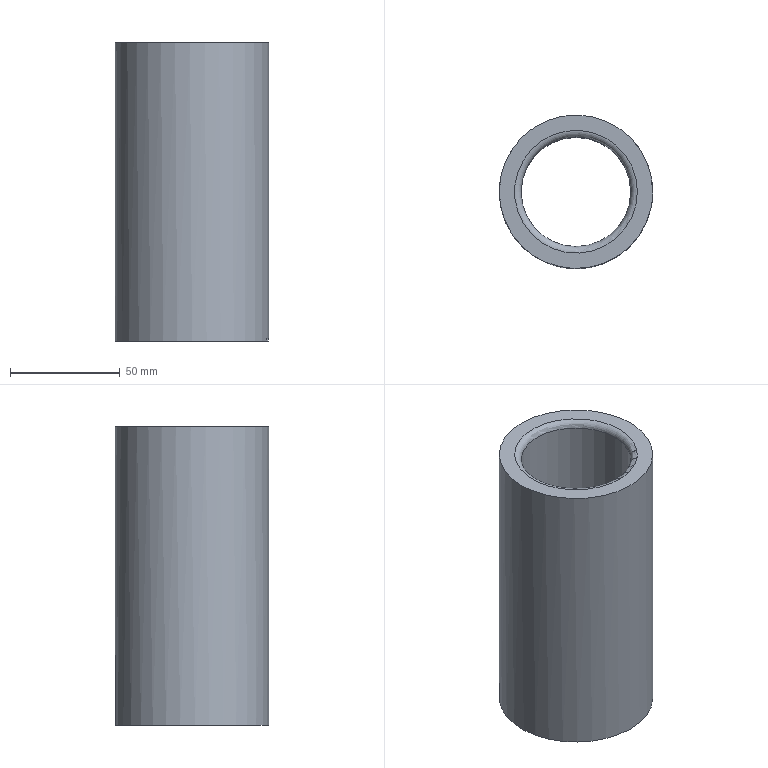Part | STEP file | solid 127 | 1 solid | 9 faces | box 70 x 70 x 136 mm | volume 255628 mm3 | plane 5 | cylinder 2 | torus 2 | commonest cylinder face diameters 50 x1 70 x1